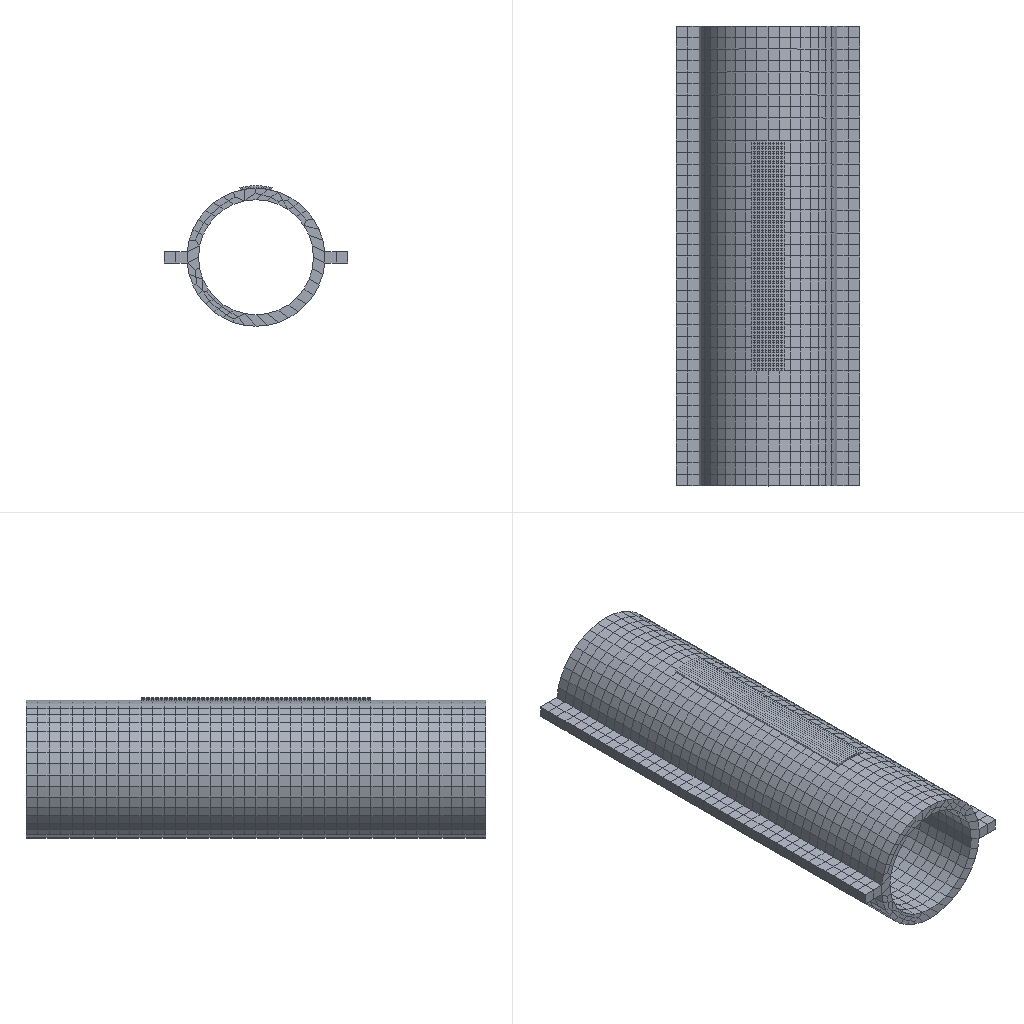Simulation study | abaqus
Set-up summary:
category,name,step,type,value,unit,region
solver,abaqus
solver,version,,,Abaqus/Standard 3DEXPERIENCE R2017x
units,not stated in the deck,,not stated
analysis,deck,,thermal,thermal
load_step,Step-delete-all,Step-delete-all,thermal,nlgeom=False
load_step,add-1,add-1,thermal,nlgeom=False
load_step,add-1-heat,add-1-heat,thermal,nlgeom=False
load_step,add-2,add-2,thermal,nlgeom=False
load_step,add-2-heat,add-2-heat,thermal,nlgeom=False
load_step,add-3,add-3,thermal,nlgeom=False
load_step,add-3-heat,add-3-heat,thermal,nlgeom=False
load_step,add-4,add-4,thermal,nlgeom=False
load_step,add-4-heat,add-4-heat,thermal,nlgeom=False
load_step,add-5,add-5,thermal,nlgeom=False
load_step,add-5-heat,add-5-heat,thermal,nlgeom=False
load_step,add-6,add-6,thermal,nlgeom=False
load_step,add-6-heat,add-6-heat,thermal,nlgeom=False
load_step,add-7,add-7,thermal,nlgeom=False
load_step,add-7-heat,add-7-heat,thermal,nlgeom=False
load_step,add-8,add-8,thermal,nlgeom=False
load_step,add-8-heat,add-8-heat,thermal,nlgeom=False
load_step,add-9,add-9,thermal,nlgeom=False
load_step,add-9-heat,add-9-heat,thermal,nlgeom=False
load_step,add-10,add-10,thermal,nlgeom=False
load_step,add-10-heat,add-10-heat,thermal,nlgeom=False
load_step,colding,colding,thermal,nlgeom=False
contact,interactions,,,general=0 pairs=0 ties=0
load_step,requested,,,22
mesh,nodes,,,6753
mesh,elements,,,3800
element_type,DC3D8,,solid,3800
load,load commands in deck,,count,12
bc,support commands in deck,,count,2
material,STEEL20G,,in results
material,INCONEL 625,,in results
check,setup vs results,,match,"per instance, exact: element labels, types and connectivity; labels of the nodes the elements use; coordinates of those nodes at SINGLE_PRECISION in 2 of 2 instance(s)"
Abaqus input file, long lists of numbers shortened:
*Heading
** Job name: Job-1 Model name: Model-1
** Generated by: Abaqus/CAE 2017
*Preprint, echo=NO, model=NO, history=NO, contact=NO
**
** PARTS
**
*Part, name=P1mm-200-100-1
*Node
      1, -0.02747,  0.15, -0.01207
      2, -0.02206,  0.15, -0.02033
** (4385 more lines like these left out)
*Element, type=DC3D8
   1,   39,    7,   49,   77,  146,  114,  156,  184
   2,   76,   48,    7,   39,  183,  155,  114,  146
** (2718 more lines like these left out)
*Nset, nset=Set-1, generate
    1,  4387,     1
*Elset, elset=Set-1, generate
    1,  2720,     1
** Section: steel20g
*Solid Section, elset=Set-1, material=steel20g
,
*End Part
**
*Part, name=P1mm-200-100-2
*Node
      1, -0.006752, 0.01, 0.02923
      2, 0.006752, 0.01, 0.02923
** (2364 more lines like these left out)
*Element, type=DC3D8
  1,   8,  93, 695, 113,   1,  45, 607,  82
  2,  93,  92, 696, 695,  45,  46, 608, 607
** (1078 more lines like these left out)
*Nset, nset=Set-1, generate
    1,  2366,     1
*Elset, elset=Set-1, generate
    1,  1080,     1
** Section: inconel625
*Solid Section, elset=Set-1, material="inconel 625"
,
*End Part
**
**
** ASSEMBLY
**
*Assembly, name=Assembly
**
*Instance, name=P1mm-200-100-1-1, part=P1mm-200-100-1
*End Instance
**
*Instance, name=P1mm-200-100-2-1, part=P1mm-200-100-2
*End Instance
**
*Nset, nset=Set-6, instance=P1mm-200-100-2-1, generate
    1,  2366,     1
*Elset, elset=Set-6, instance=P1mm-200-100-2-1, generate
    1,  1080,     1
*Nset, nset=Set-7, instance=P1mm-200-100-2-1
   35,   36,   38,   39,   41,   42,   43,   44,  464,  465,  466,  467,  468,  469,  470,  471
  472,  473,  474,  502,  503,  504,  505,  506,  507,  508,  509,  510,  511,  512,  553,  554
** (15 more lines like these left out)
*Elset, elset=Set-7, instance=P1mm-200-100-2-1, generate
  973,  1080,     1
*Nset, nset=Set-8, instance=P1mm-200-100-2-1
   33,   34,   35,   36,   37,   38,   39,   40,  445,  446,  447,  448,  449,  450,  451,  452
  453,  454,  455,  456,  457,  458,  459,  460,  461,  462,  463,  464,  465,  466,  467,  468
** (15 more lines like these left out)
*Elset, elset=Set-8, instance=P1mm-200-100-2-1, generate
 757,  864,    1
*Nset, nset=Set-9, instance=P1mm-200-100-2-1
   27,   28,   30,   31,   33,   34,   37,   40,  356,  357,  358,  359,  360,  361,  362,  363
  364,  365,  366,  394,  395,  396,  397,  398,  399,  400,  401,  402,  403,  404,  445,  446
** (15 more lines like these left out)
*Elset, elset=Set-9, instance=P1mm-200-100-2-1, generate
 865,  972,    1
*Nset, nset=Set-10, instance=P1mm-200-100-2-1
   25,   26,   27,   28,   29,   30,   31,   32,  337,  338,  339,  340,  341,  342,  343,  344
  345,  346,  347,  348,  349,  350,  351,  352,  353,  354,  355,  356,  357,  358,  359,  360
** (15 more lines like these left out)
*Elset, elset=Set-10, instance=P1mm-200-100-2-1, generate
 541,  648,    1
*Nset, nset=Set-11, instance=P1mm-200-100-2-1
   19,   20,   22,   23,   25,   26,   29,   32,  248,  249,  250,  251,  252,  253,  254,  255
  256,  257,  258,  286,  287,  288,  289,  290,  291,  292,  293,  294,  295,  296,  337,  338
** (15 more lines like these left out)
*Elset, elset=Set-11, instance=P1mm-200-100-2-1, generate
 649,  756,    1
*Nset, nset=Set-12, instance=P1mm-200-100-2-1
   17,   18,   19,   20,   21,   22,   23,   24,  229,  230,  231,  232,  233,  234,  235,  236
  237,  238,  239,  240,  241,  242,  243,  244,  245,  246,  247,  248,  249,  250,  251,  252
** (15 more lines like these left out)
*Elset, elset=Set-12, instance=P1mm-200-100-2-1, generate
 325,  432,    1
*Nset, nset=Set-13, instance=P1mm-200-100-2-1
   11,   12,   14,   15,   17,   18,   21,   24,  140,  141,  142,  143,  144,  145,  146,  147
  148,  149,  150,  178,  179,  180,  181,  182,  183,  184,  185,  186,  187,  188,  229,  230
** (15 more lines like these left out)
*Elset, elset=Set-13, instance=P1mm-200-100-2-1, generate
 433,  540,    1
*Nset, nset=Set-14, instance=P1mm-200-100-2-1
   9,  10,  11,  12,  13,  14,  15,  16, 121, 122, 123, 124, 125, 126, 127, 128
 129, 130, 131, 132, 133, 134, 135, 136, 137, 138, 139, 140, 141, 142, 143, 144
** (15 more lines like these left out)
*Elset, elset=Set-14, instance=P1mm-200-100-2-1, generate
 109,  216,    1
*Nset, nset=Set-15, instance=P1mm-200-100-2-1
    1,    2,    5,    8,    9,   10,   13,   16,   45,   46,   47,   48,   49,   50,   51,   52
   53,   54,   55,   83,   84,   85,   86,   87,   88,   89,   90,   91,   92,   93,  121,  122
** (15 more lines like these left out)
*Elset, elset=Set-15, instance=P1mm-200-100-2-1, generate
 217,  324,    1
*Nset, nset=Set-16, instance=P1mm-200-100-2-1
   1,   2,   3,   4,   5,   6,   7,   8,  45,  46,  47,  48,  49,  50,  51,  52
  53,  54,  55,  56,  57,  58,  59,  60,  61,  62,  63,  64,  65,  66,  67,  68
** (15 more lines like these left out)
*Elset, elset=Set-16, instance=P1mm-200-100-2-1, generate
   1,  108,    1
*Nset, nset=Set-17, instance=P1mm-200-100-2-1
   1,   2,   3,   4,   5,   6,   7,   8,  45,  46,  47,  48,  49,  50,  51,  52
  53,  54,  55,  56,  57,  58,  59,  60,  61,  62,  63,  64,  65,  66,  67,  68
** (15 more lines like these left out)
*Elset, elset=Set-17, instance=P1mm-200-100-2-1, generate
   1,  108,    1
*Nset, nset=Set-18, instance=P1mm-200-100-2-1
    1,    2,    5,    8,    9,   10,   13,   16,   45,   46,   47,   48,   49,   50,   51,   52
   53,   54,   55,   83,   84,   85,   86,   87,   88,   89,   90,   91,   92,   93,  121,  122
** (15 more lines like these left out)
*Elset, elset=Set-18, instance=P1mm-200-100-2-1, generate
 217,  324,    1
*Nset, nset=Set-19, instance=P1mm-200-100-2-1
   9,  10,  11,  12,  13,  14,  15,  16, 121, 122, 123, 124, 125, 126, 127, 128
 129, 130, 131, 132, 133, 134, 135, 136, 137, 138, 139, 140, 141, 142, 143, 144
** (15 more lines like these left out)
*Elset, elset=Set-19, instance=P1mm-200-100-2-1, generate
 109,  216,    1
*Nset, nset=Set-20, instance=P1mm-200-100-2-1
   11,   12,   14,   15,   17,   18,   21,   24,  140,  141,  142,  143,  144,  145,  146,  147
  148,  149,  150,  178,  179,  180,  181,  182,  183,  184,  185,  186,  187,  188,  229,  230
** (15 more lines like these left out)
*Elset, elset=Set-20, instance=P1mm-200-100-2-1, generate
 433,  540,    1
*Nset, nset=Set-21, instance=P1mm-200-100-2-1
   17,   18,   19,   20,   21,   22,   23,   24,  229,  230,  231,  232,  233,  234,  235,  236
  237,  238,  239,  240,  241,  242,  243,  244,  245,  246,  247,  248,  249,  250,  251,  252
** (15 more lines like these left out)
*Elset, elset=Set-21, instance=P1mm-200-100-2-1, generate
 325,  432,    1
*Nset, nset=Set-22, instance=P1mm-200-100-2-1
   19,   20,   22,   23,   25,   26,   29,   32,  248,  249,  250,  251,  252,  253,  254,  255
  256,  257,  258,  286,  287,  288,  289,  290,  291,  292,  293,  294,  295,  296,  337,  338
** (15 more lines like these left out)
*Elset, elset=Set-22, instance=P1mm-200-100-2-1, generate
 649,  756,    1
*Nset, nset=Set-23, instance=P1mm-200-100-2-1
   25,   26,   27,   28,   29,   30,   31,   32,  337,  338,  339,  340,  341,  342,  343,  344
  345,  346,  347,  348,  349,  350,  351,  352,  353,  354,  355,  356,  357,  358,  359,  360
** (15 more lines like these left out)
*Elset, elset=Set-23, instance=P1mm-200-100-2-1, generate
 541,  648,    1
*Nset, nset=Set-24, instance=P1mm-200-100-2-1
   27,   28,   30,   31,   33,   34,   37,   40,  356,  357,  358,  359,  360,  361,  362,  363
  364,  365,  366,  394,  395,  396,  397,  398,  399,  400,  401,  402,  403,  404,  445,  446
** (15 more lines like these left out)
*Elset, elset=Set-24, instance=P1mm-200-100-2-1, generate
 865,  972,    1
*Nset, nset=Set-25, instance=P1mm-200-100-2-1
   33,   34,   35,   36,   37,   38,   39,   40,  445,  446,  447,  448,  449,  450,  451,  452
  453,  454,  455,  456,  457,  458,  459,  460,  461,  462,  463,  464,  465,  466,  467,  468
** (15 more lines like these left out)
*Elset, elset=Set-25, instance=P1mm-200-100-2-1, generate
 757,  864,    1
*Nset, nset=Set-26, instance=P1mm-200-100-2-1
   35,   36,   38,   39,   41,   42,   43,   44,  464,  465,  466,  467,  468,  469,  470,  471
  472,  473,  474,  502,  503,  504,  505,  506,  507,  508,  509,  510,  511,  512,  553,  554
** (15 more lines like these left out)
*Elset, elset=Set-26, instance=P1mm-200-100-2-1, generate
  973,  1080,     1
*Elset, elset=_Surf-5_S2, internal, instance=P1mm-200-100-2-1, generate
   1,  108,    1
*Elset, elset=_Surf-5_S4, internal, instance=P1mm-200-100-2-1, generate
  12,  108,   12
*Elset, elset=_Surf-5_S1, internal, instance=P1mm-200-100-2-1, generate
   1,  108,    1
*Elset, elset=_Surf-5_S5, internal, instance=P1mm-200-100-2-1, generate
  97,  108,    1
*Surface, type=ELEMENT, name=Surf-5
_Surf-5_S2, S2
_Surf-5_S4, S4
_Surf-5_S1, S1
_Surf-5_S5, S5
*Elset, elset=_Surf-6_S2, internal, instance=P1mm-200-100-2-1, generate
    1,  1080,     1
*Elset, elset=_Surf-6_S4, internal, instance=P1mm-200-100-2-1, generate
   12,  1080,    12
*Elset, elset=_Surf-6_S1, internal, instance=P1mm-200-100-2-1, generate
    1,  1080,     1
*Elset, elset=_Surf-6_S6, internal, instance=P1mm-200-100-2-1, generate
    1,  1069,    12
*Elset, elset=_Surf-6_S5, internal, instance=P1mm-200-100-2-1
   97,   98,   99,  100,  101,  102,  103,  104,  105,  106,  107,  108, 1069, 1070, 1071, 1072
 1073, 1074, 1075, 1076, 1077, 1078, 1079, 1080
*Surface, type=ELEMENT, name=Surf-6
_Surf-6_S2, S2
_Surf-6_S4, S4
_Surf-6_S6, S6
_Surf-6_S1, S1
_Surf-6_S5, S5
*Elset, elset=_Surf-7_S2, internal, instance=P1mm-200-100-2-1, generate
    1,  1080,     1
*Elset, elset=_Surf-7_S4, internal, instance=P1mm-200-100-2-1, generate
   12,  1080,    12
*Elset, elset=_Surf-7_S1, internal, instance=P1mm-200-100-2-1, generate
    1,  1080,     1
*Elset, elset=_Surf-7_S6, internal, instance=P1mm-200-100-2-1, generate
    1,  1069,    12
*Elset, elset=_Surf-7_S5, internal, instance=P1mm-200-100-2-1
   97,   98,   99,  100,  101,  102,  103,  104,  105,  106,  107,  108, 1069, 1070, 1071, 1072
 1073, 1074, 1075, 1076, 1077, 1078, 1079, 1080
*Surface, type=ELEMENT, name=Surf-7
_Surf-7_S2, S2
_Surf-7_S4, S4
_Surf-7_S6, S6
_Surf-7_S1, S1
_Surf-7_S5, S5
*End Assembly
**
** MATERIALS
**
*Material, name="inconel 625"
*Conductivity
10., 21.
11., 93.
13.,204.
13.,316.
14.,427.
16.,538.
18.,649.
19.,760.
21.,871.
25.,937.
*Density
8400.,
*Elastic
 2.075e+11, 0.278,   21.
 2.041e+11,  0.28,   93.
 1.979e+11, 0.286,  204.
 1.917e+11,  0.29,  316.
 1.856e+11, 0.295,  427.
 1.786e+11, 0.312,  538.
 1.703e+11, 0.314,  649.
 1.606e+11, 0.305,  760.
 1.475e+11, 0.289,  871.
*Expansion
 1.28e-05, 93.
 1.31e-05,204.
 1.33e-05,316.
 1.37e-05,427.
  1.4e-05,538.
 1.48e-05,649.
 1.53e-05,760.
 1.58e-05,871.
 1.62e-05,937.
*Plastic
 4.35e+08,      0.,     21.
 3.76e+08,  0.0001,     93.
 3.58e+08,  0.0002,    204.
  3.5e+08,  0.0003,    316.
 3.35e+08,  0.0004,    427.
  3.2e+08, 0.00051,    538.
 2.75e+08, 0.00052,    649.
 2.44e+08, 0.00053,    760.
 1.83e+08, 0.00054,    871.
 1.66e+08, 0.00055,    937.
  9.5e+07, 0.00056,   1093.
*Specific Heat
410.,  21.
425.,  93.
456., 204.
481., 316.
511., 427.
536., 538.
565., 649.
590., 760.
620., 871.
645., 937.
670.,1093.
*Material, name=steel20g
*Conductivity
 5.234,  20.
 4.857, 200.
 3.768, 500.
 2.763, 800.
 2.234,1000.
 1.629,1300.
 1.238,1400.
*Density
7850.,
*Elastic
 2.09e+11, 0.3, 20.
 1.97e+11, 0.3,100.
 1.74e+11, 0.3,200.
  4.3e+11, 0.3,300.
  2.2e+11, 0.3,400.
    2e+11, 0.3,500.
  1.3e+11, 0.3,600.
*Expansion
 1.49e-05,  20.
 1.28e-05, 200.
 1.42e-05, 500.
 1.49e-05, 800.
 1.46e-05,1000.
 1.44e-05,1300.
  1.9e-05,1400.
*Plastic
 2.78e+08,     0.,    20.
 1.83e+08, 0.0001,   200.
 1.59e+08, 0.0002,   500.
  7.7e+07, 0.0003,   800.
  4.6e+07, 0.0004,  1000.
  2.3e+07, 0.0005,  1300.
  1.6e+07,  6e-05,  1400.
*Specific Heat
460.,  20.
498., 200.
578., 500.
659., 800.
695.,1000.
687.,1300.
648.,1400.
**
** PHYSICAL CONSTANTS
**
*Physical Constants, absolute zero=-273.13, stefan boltzmann=5.67e-08
** ----------------------------------------------------------------
**
** [REDACTED] : [REDACTED] -delete-all
**
*Step, name=Step-delete-all, nlgeom=NO
*Heat Transfer, end=PERIOD, deltmx=100000.
1., 1., 1e-05, 1.,
**
** INTERACTIONS
**
** Interaction: Int-1
*Model Change, remove
Set-6,
**
** OUTPUT REQUESTS
**
*Restart, write, frequency=0
*Output, field, frequency=0
*Output, history, frequency=0
*End Step
** ----------------------------------------------------------------
**
** [REDACTED] : add-1
**
*Step, name=add-1, nlgeom=NO, inc=1000
*Heat Transfer, end=PERIOD, deltmx=10000.
0.001, 0.6, 6e-06, 0.1,
**
** INTERACTIONS
**
** Interaction: add1
*Model Change, add
Set-7,
**
** OUTPUT REQUESTS
**
*Restart, write, frequency=0
**
** FIELD OUTPUT: F-Output-1
**
*Output, field
*Node Output
NT, RFL
*Element Output, directions=YES
HFL, TEMP
*Output, history, frequency=0
*End Step
** ----------------------------------------------------------------
**
** [REDACTED] : add-1-heat
**
*Step, name=add-1-heat, nlgeom=NO
*Heat Transfer, end=PERIOD, deltmx=10000.
0.6, 0.6, 6e-06, 0.6,
**
** LOADS
**
** Name: Load-1   Type: Body heat flux
*Dflux
Set-17, BFNU, 1.
**
** INTERACTIONS
**
** Interaction: c1
*Sfilm
Surf-6, F, 20., 0.8
** Interaction: c2
*Sradiate
Surf-7, R, 20., 0.2
**
** OUTPUT REQUESTS
**
*Restart, write, frequency=0
**
** FIELD OUTPUT: F-Output-1
**
*Output, field
*Node Output
NT, RFL
*Element Output, directions=YES
HFL, TEMP
*Output, history, frequency=0
*End Step
** ----------------------------------------------------------------
**
** [REDACTED] : add-2
**
*Step, name=add-2, nlgeom=NO
*Heat Transfer, end=PERIOD, deltmx=100000.
1.2, 1.2, 1.2e-05, 1.2,
**
** LOADS
**
** Name: Load-1   Type: Body heat flux
*Dflux, op=NEW
**
** INTERACTIONS
**
** Interaction: add2
*Model Change, add
Set-8,
**
** OUTPUT REQUESTS
**
*Restart, write, frequency=0
**
** FIELD OUTPUT: F-Output-1
**
*Output, field
*Node Output
NT, RFL
*Element Output, directions=YES
HFL, TEMP
*Output, history, frequency=0
*End Step
** ----------------------------------------------------------------
**
** [REDACTED] : add-2-heat
**
*Step, name=add-2-heat, nlgeom=NO
*Heat Transfer, end=PERIOD, deltmx=10000.
1.2, 1.2, 1.2e-05, 1.2,
**
** LOADS
**
** Name: Load-2   Type: Body heat flux
*Dflux
Set-18, BFNU, 1.
**
** OUTPUT REQUESTS
**
*Restart, write, frequency=0
**
** FIELD OUTPUT: F-Output-1
**
*Output, field
*Node Output
NT, RFL
*Element Output, directions=YES
HFL, TEMP
*Output, history, frequency=0
*End Step
** ----------------------------------------------------------------
**
** [REDACTED] : add-3
**
*Step, name=add-3, nlgeom=NO
*Heat Transfer, end=PERIOD, deltmx=1e+07
1.8, 1.8, 1.8e-05, 1.8,
**
** LOADS
**
** Name: Load-2   Type: Body heat flux
*Dflux, op=NEW
**
** INTERACTIONS
**
** Interaction: add3
*Model Change, add
Set-9,
**
** OUTPUT REQUESTS
**
*Restart, write, frequency=0
**
** FIELD OUTPUT: F-Output-1
**
*Output, field
*Node Output
NT, RFL
*Element Output, directions=YES
HFL, TEMP
*Output, history, frequency=0
*End Step
** ----------------------------------------------------------------
**
** [REDACTED] : add-3-heat
**
*Step, name=add-3-heat, nlgeom=NO
*Heat Transfer, end=PERIOD, deltmx=10000.
1.8, 1.8, 1.8e-05, 1.8,
**
** LOADS
**
** Name: Load-3   Type: Body heat flux
*Dflux
Set-19, BFNU, 1.
**
** OUTPUT REQUESTS
**
*Restart, write, frequency=0
**
** FIELD OUTPUT: F-Output-1
**
*Output, field
*Node Output
NT, RFL
*Element Output, directions=YES
HFL, TEMP
*Output, history, frequency=0
*End Step
** ----------------------------------------------------------------
**
** [REDACTED] : add-4
**
*Step, name=add-4, nlgeom=NO
*Heat Transfer, end=PERIOD, deltmx=100000.
2.4, 2.4, 2.4e-05, 2.4,
**
** LOADS
**
** Name: Load-3   Type: Body heat flux
*Dflux, op=NEW
**
** INTERACTIONS
**
** Interaction: add4
*Model Change, add
Set-10,
**
** OUTPUT REQUESTS
**
*Restart, write, frequency=0
**
** FIELD OUTPUT: F-Output-1
**
*Output, field
*Node Output
NT, RFL
*Element Output, directions=YES
HFL, TEMP
*Output, history, frequency=0
*End Step
** ----------------------------------------------------------------
**
** [REDACTED] : add-4-heat
**
*Step, name=add-4-heat, nlgeom=NO
*Heat Transfer, end=PERIOD, deltmx=10000.
2.4, 2.4, 2.4e-05, 2.4,
**
** LOADS
**
** Name: Load-4   Type: Body heat flux
*Dflux
Set-20, BFNU, 1.
**
** OUTPUT REQUESTS
**
*Restart, write, frequency=0
**
** FIELD OUTPUT: F-Output-1
**
*Output, field
*Node Output
NT, RFL
*Element Output, directions=YES
HFL, TEMP
*Output, history, frequency=0
*End Step
** ----------------------------------------------------------------
**
** [REDACTED] : add-5
**
*Step, name=add-5, nlgeom=NO
*Heat Transfer, end=PERIOD, deltmx=10000.
3., 3., 3e-05, 3.,
**
** LOADS
**
** Name: Load-4   Type: Body heat flux
*Dflux, op=NEW
**
** INTERACTIONS
**
** Interaction: add5
*Model Change, add
Set-11,
**
** OUTPUT REQUESTS
**
*Restart, write, frequency=0
**
** FIELD OUTPUT: F-Output-1
**
*Output, field
*Node Output
NT, RFL
*Element Output, directions=YES
HFL, TEMP
*Output, history, frequency=0
*End Step
** ----------------------------------------------------------------
**
** [REDACTED] : add-5-heat
**
*Step, name=add-5-heat, nlgeom=NO
*Heat Transfer, end=PERIOD, deltmx=10000.
3., 3., 3e-05, 3.,
**
** LOADS
**
** Name: Load-5   Type: Body heat flux
*Dflux
Set-21, BFNU, 1.
**
** OUTPUT REQUESTS
**
*Restart, write, frequency=0
**
** FIELD OUTPUT: F-Output-1
**
*Output, field
*Node Output
NT, RFL
*Element Output, directions=YES
HFL, TEMP
*Output, history, frequency=0
*End Step
** ----------------------------------------------------------------
**
** [REDACTED] : add-6
**
*Step, name=add-6, nlgeom=NO
*Heat Transfer, end=PERIOD, deltmx=1e+06
3.6, 3.6, 3.6e-05, 3.6,
**
** LOADS
**
** Name: Load-5   Type: Body heat flux
*Dflux, op=NEW
**
** INTERACTIONS
**
** Interaction: add6
*Model Change, add
Set-12,
**
** OUTPUT REQUESTS
**
*Restart, write, frequency=0
**
** FIELD OUTPUT: F-Output-1
**
*Output, field
*Node Output
NT, RFL
*Element Output, directions=YES
HFL, TEMP
*Output, history, frequency=0
*End Step
** ----------------------------------------------------------------
**
** [REDACTED] : add-6-heat
**
*Step, name=add-6-heat, nlgeom=NO
*Heat Transfer, end=PERIOD, deltmx=10000.
3.6, 3.6, 3.6e-05, 3.6,
**
** LOADS
**
** Name: Load-6   Type: Body heat flux
*Dflux
Set-22, BFNU, 1.
**
** OUTPUT REQUESTS
**
*Restart, write, frequency=0
**
** FIELD OUTPUT: F-Output-1
**
*Output, field
*Node Output
NT, RFL
*Element Output, directions=YES
HFL, TEMP
*Output, history, frequency=0
*End Step
** ----------------------------------------------------------------
**
** [REDACTED] : add-7
**
*Step, name=add-7, nlgeom=NO
*Heat Transfer, end=PERIOD, deltmx=10000.
4.2, 4.2, 4.2e-05, 4.2,
**
** LOADS
**
** Name: Load-6   Type: Body heat flux
*Dflux, op=NEW
**
** INTERACTIONS
**
** Interaction: add7
*Model Change, add
Set-13,
**
** OUTPUT REQUESTS
**
*Restart, write, frequency=0
**
** FIELD OUTPUT: F-Output-1
**
*Output, field
*Node Output
NT, RFL
*Element Output, directions=YES
HFL, TEMP
*Output, history, frequency=0
*End Step
** ----------------------------------------------------------------
**
** [REDACTED] : add-7-heat
**
*Step, name=add-7-heat, nlgeom=NO
*Heat Transfer, end=PERIOD, deltmx=10000.
4.2, 4.2, 4.2e-05, 4.2,
**
** LOADS
**
** Name: Load-7   Type: Body heat flux
*Dflux
Set-23, BFNU, 1.
**
** OUTPUT REQUESTS
**
*Restart, write, frequency=0
**
** FIELD OUTPUT: F-Output-1
**
*Output, field
*Node Output
NT, RFL
*Element Output, directions=YES
HFL, TEMP
*Output, history, frequency=0
*End Step
** ----------------------------------------------------------------
**
** [REDACTED] : add-8
**
*Step, name=add-8, nlgeom=NO
*Heat Transfer, end=PERIOD, deltmx=10000.
4.8, 4.8, 4.8e-05, 4.8,
**
** LOADS
**
** Name: Load-7   Type: Body heat flux
*Dflux, op=NEW
**
** INTERACTIONS
**
** Interaction: add8
*Model Change, add
Set-14,
**
** OUTPUT REQUESTS
**
*Restart, write, frequency=0
**
** FIELD OUTPUT: F-Output-1
**
*Output, field
*Node Output
NT, RFL
*Element Output, directions=YES
HFL, TEMP
*Output, history, frequency=0
*End Step
** ----------------------------------------------------------------
**
** [REDACTED] : add-8-heat
**
*Step, name=add-8-heat, nlgeom=NO
*Heat Transfer, end=PERIOD, deltmx=10000.
4.8, 4.8, 4.8e-05, 4.8,
**
** LOADS
**
** Name: Load-8   Type: Body heat flux
*Dflux
Set-24, BFNU, 1.
**
** OUTPUT REQUESTS
**
*Restart, write, frequency=0
**
** FIELD OUTPUT: F-Output-1
**
*Output, field
*Node Output
NT, RFL
*Element Output, directions=YES
HFL, TEMP
*Output, history, frequency=0
*End Step
** ----------------------------------------------------------------
**
** [REDACTED] : add-9
**
*Step, name=add-9, nlgeom=NO
*Heat Transfer, end=PERIOD, deltmx=10000.
5.4, 5.4, 5.4e-05, 5.4,
**
** LOADS
**
** Name: Load-8   Type: Body heat flux
*Dflux, op=NEW
**
** INTERACTIONS
**
** Interaction: add9
*Model Change, add
Set-15,
**
** OUTPUT REQUESTS
**
*Restart, write, frequency=0
**
** FIELD OUTPUT: F-Output-1
**
*Output, field
*Node Output
NT, RFL
*Element Output, directions=YES
HFL, TEMP
*Output, history, frequency=0
*End Step
** ----------------------------------------------------------------
**
** [REDACTED] : add-9-heat
**
*Step, name=add-9-heat, nlgeom=NO
*Heat Transfer, end=PERIOD, deltmx=10000.
5.4, 5.4, 5.4e-05, 5.4,
**
** LOADS
**
** Name: Load-9   Type: Body heat flux
*Dflux
Set-25, BFNU, 1.
**
** OUTPUT REQUESTS
**
*Restart, write, frequency=0
**
** FIELD OUTPUT: F-Output-1
**
*Output, field
*Node Output
NT, RFL
*Element Output, directions=YES
HFL, TEMP
*Output, history, frequency=0
*End Step
** ----------------------------------------------------------------
**
** [REDACTED] : add-10
**
*Step, name=add-10, nlgeom=NO
*Heat Transfer, end=PERIOD, deltmx=10000.
6., 6., 6e-05, 6.,
**
** LOADS
**
** Name: Load-9   Type: Body heat flux
*Dflux, op=NEW
**
** INTERACTIONS
**
** Interaction: add10
*Model Change, add
Set-16,
**
** OUTPUT REQUESTS
**
*Restart, write, frequency=0
**
** FIELD OUTPUT: F-Output-1
**
*Output, field
*Node Output
NT, RFL
*Element Output, directions=YES
HFL, TEMP
*Output, history, frequency=0
*End Step
** ----------------------------------------------------------------
**
** [REDACTED] : add-10-heat
**
*Step, name=add-10-heat, nlgeom=NO
*Heat Transfer, end=PERIOD, deltmx=1000.
6., 6., 6e-05, 6.,
**
** LOADS
**
** Name: Load-10   Type: Body heat flux
*Dflux
Set-26, BFNU, 1.
**
** OUTPUT REQUESTS
**
*Restart, write, frequency=0
**
** FIELD OUTPUT: F-Output-1
**
*Output, field
*Node Output
NT, RFL
*Element Output, directions=YES
HFL, TEMP
*Output, history, frequency=0
*End Step
** ----------------------------------------------------------------
**
** [REDACTED] : colding
**
*Step, name=colding, nlgeom=NO, inc=1000000
*Heat Transfer, end=PERIOD, deltmx=100000.
0.1, 500., 0.005, 1.,
**
** LOADS
**
** Name: Load-10   Type: Body heat flux
*Dflux, op=NEW
**
** OUTPUT REQUESTS
**
*Restart, write, frequency=0
**
** FIELD OUTPUT: F-Output-1
**
*Output, field
*Node Output
NT, RFL
*Element Output, directions=YES
HFL, TEMP
*Output, history, frequency=0
*End Step
Results summary:
result,step,,partial,increments=0 time=0.0/1.0
result,step,,partial,increments=0 time=0.0/0.6
result,step,,partial,increments=0 time=0.0/0.6
result,step,,partial,increments=0 time=0.0/1.2
result,step,,partial,increments=0 time=0.0/1.2
result,step,,partial,increments=0 time=0.0/1.8
result,step,,partial,increments=0 time=0.0/1.8
result,step,,partial,increments=0 time=0.0/2.4
result,step,,partial,increments=0 time=0.0/2.4
result,step,,partial,increments=0 time=0.0/3.0
result,step,,partial,increments=0 time=0.0/3.0
result,step,,partial,increments=0 time=0.0/3.6
result,step,,partial,increments=0 time=0.0/3.6
result,step,,partial,increments=0 time=0.0/4.2
result,step,,partial,increments=0 time=0.0/4.2
result,step,,partial,increments=0 time=0.0/4.8
result,step,,partial,increments=0 time=0.0/4.8
result,step,,partial,increments=0 time=0.0/5.4
result,step,,partial,increments=0 time=0.0/5.4
result,step,,partial,increments=0 time=0.0/6.0
result,step,,partial,increments=0 time=0.0/6.0
result,step,,partial,increments=0 time=0.0/500.0
result,analysis,,,"heat transfer, deltamx"
result,last_loadstep,,,21
result,analysis steps,,count,22
result,primary field,,,NT11